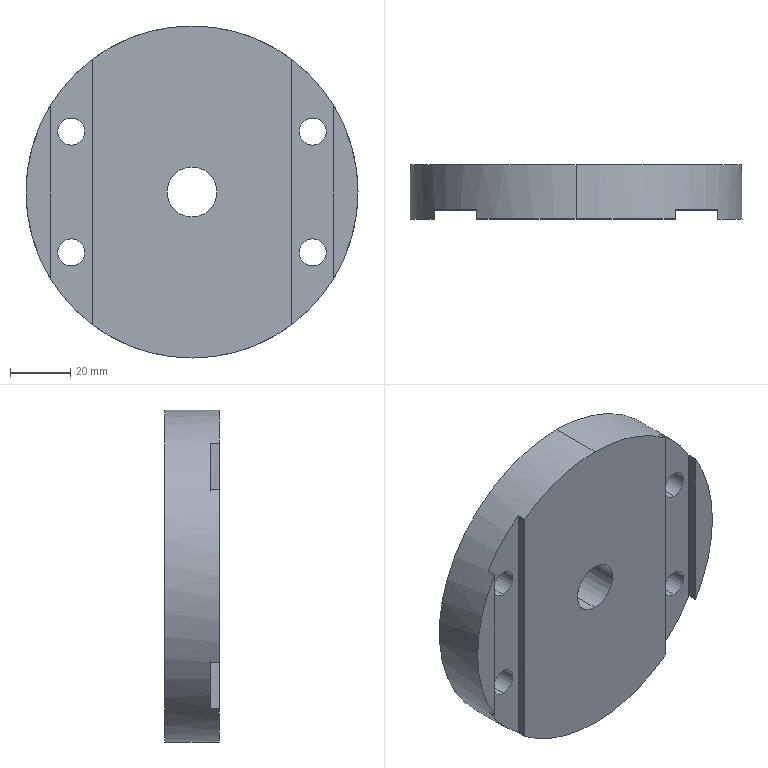Part | STEP file | 1 solid | 34 faces | box 110 x 18 x 110 mm | volume 153241 mm3 | cylinder 20 | plane 14 | commonest cylinder face diameters 9 x8 15 x8 16.5 x2 110 x2